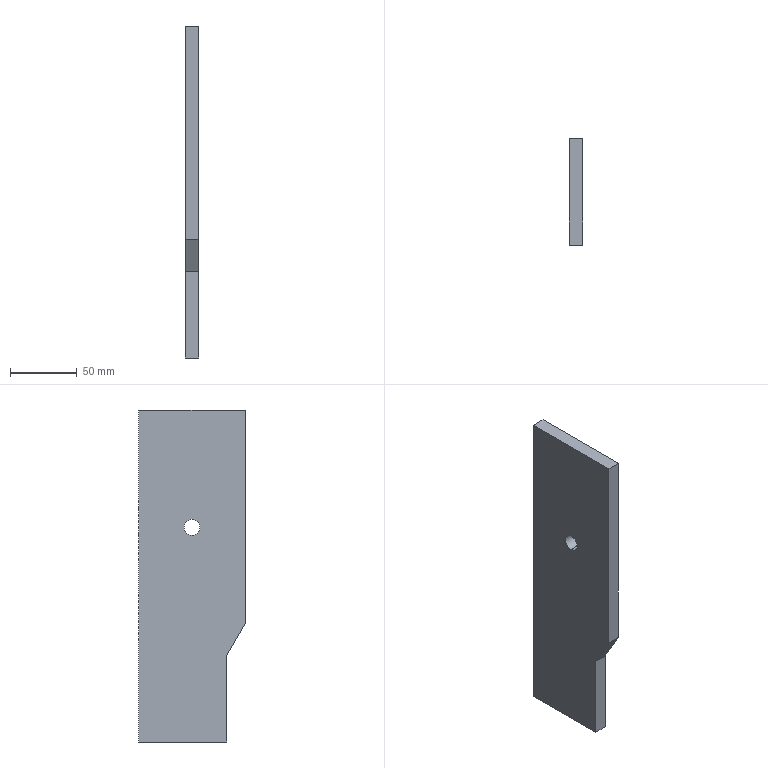Part | STEP file | VD-SYL0380DJ1006_1_4-3_VD-SYL03 | 1 solid | 10 faces | box 10 x 80 x 249 mm | volume 187272 mm3 | plane 8 | cylinder 2 | commonest cylinder face diameters 12 x2
STEP:
#1=CARTESIAN_POINT('',(0.,-40.,-94.));
#2=VERTEX_POINT('',#1);
#3=CARTESIAN_POINT('',(10.,-40.,-94.));
#4=VERTEX_POINT('',#3);
#5=CARTESIAN_POINT('',(0.,-40.,-94.));
#6=DIRECTION('',(1.,0.,0.));
#7=VECTOR('',#6,1000.);
#8=LINE('',#5,#7);
#9=EDGE_CURVE('',#2,#4,#8,.T.);
#10=ORIENTED_EDGE('',*,*,#9,.F.);
#11=CARTESIAN_POINT('',(0.,-40.,-82.));
#12=VERTEX_POINT('',#11);
#13=CARTESIAN_POINT('',(0.,-40.,-88.));
#14=DIRECTION('',(1.,0.,0.));
#15=DIRECTION('',(0.,0.,1.));
#16=AXIS2_PLACEMENT_3D('',#13,#14,#15);
#17=CIRCLE('',#16,6.);
#18=EDGE_CURVE('',#12,#2,#17,.T.);
#19=ORIENTED_EDGE('',*,*,#18,.F.);
#20=CARTESIAN_POINT('',(10.,-40.,-82.));
#21=VERTEX_POINT('',#20);
#22=CARTESIAN_POINT('',(0.,-40.,-82.));
#23=DIRECTION('',(1.,0.,0.));
#24=VECTOR('',#23,1000.);
#25=LINE('',#22,#24);
#26=EDGE_CURVE('',#12,#21,#25,.T.);
#27=ORIENTED_EDGE('',*,*,#26,.T.);
#28=CARTESIAN_POINT('',(10.,-40.,-88.));
#29=DIRECTION('',(-1.,0.,0.));
#30=DIRECTION('',(0.,0.,-1.));
#31=AXIS2_PLACEMENT_3D('',#28,#29,#30);
#32=CIRCLE('',#31,6.);
#33=EDGE_CURVE('',#4,#21,#32,.T.);
#34=ORIENTED_EDGE('',*,*,#33,.F.);
#35=EDGE_LOOP('',(#10,#19,#27,#34));
#36=FACE_OUTER_BOUND('',#35,.T.);
#37=CARTESIAN_POINT('',(0.,-40.,-88.));
#38=DIRECTION('',(-1.,0.,0.));
#39=DIRECTION('',(0.,0.,1.));
#40=AXIS2_PLACEMENT_3D('',#37,#38,#39);
#41=CYLINDRICAL_SURFACE('',#40,6.);
#42=ADVANCED_FACE('',(#36),#41,.F.);
#43=CARTESIAN_POINT('',(10.,-40.,-88.));
#44=DIRECTION('',(-1.,0.,0.));
#45=DIRECTION('',(0.,0.,1.));
#46=AXIS2_PLACEMENT_3D('',#43,#44,#45);
#47=CIRCLE('',#46,6.);
#48=EDGE_CURVE('',#21,#4,#47,.T.);
#49=ORIENTED_EDGE('',*,*,#48,.F.);
#50=ORIENTED_EDGE('',*,*,#26,.F.);
#51=CARTESIAN_POINT('',(0.,-40.,-88.));
#52=DIRECTION('',(1.,0.,0.));
#53=DIRECTION('',(0.,0.,-1.));
#54=AXIS2_PLACEMENT_3D('',#51,#52,#53);
#55=CIRCLE('',#54,6.);
#56=EDGE_CURVE('',#2,#12,#55,.T.);
#57=ORIENTED_EDGE('',*,*,#56,.F.);
#58=ORIENTED_EDGE('',*,*,#9,.T.);
#59=EDGE_LOOP('',(#49,#50,#57,#58));
#60=FACE_OUTER_BOUND('',#59,.T.);
#61=CARTESIAN_POINT('',(0.,-40.,-88.));
#62=DIRECTION('',(-1.,0.,0.));
#63=DIRECTION('',(0.,0.,1.));
#64=AXIS2_PLACEMENT_3D('',#61,#62,#63);
#65=CYLINDRICAL_SURFACE('',#64,6.);
#66=ADVANCED_FACE('',(#60),#65,.F.);
#67=ORIENTED_EDGE('',*,*,#33,.T.);
#68=ORIENTED_EDGE('',*,*,#48,.T.);
#69=EDGE_LOOP('',(#67,#68));
#70=FACE_BOUND('',#69,.T.);
#71=CARTESIAN_POINT('',(10.,0.,0.));
#72=VERTEX_POINT('',#71);
#73=CARTESIAN_POINT('',(10.,0.,-249.));
#74=VERTEX_POINT('',#73);
#75=CARTESIAN_POINT('',(10.,0.,0.));
#76=DIRECTION('',(0.,0.,-1.));
#77=VECTOR('',#76,1000.);
#78=LINE('',#75,#77);
#79=EDGE_CURVE('',#72,#74,#78,.T.);
#80=ORIENTED_EDGE('',*,*,#79,.F.);
#81=CARTESIAN_POINT('',(10.,-80.,0.));
#82=VERTEX_POINT('',#81);
#83=CARTESIAN_POINT('',(10.,-80.,0.));
#84=DIRECTION('',(0.,1.,0.));
#85=VECTOR('',#84,1000.);
#86=LINE('',#83,#85);
#87=EDGE_CURVE('',#82,#72,#86,.T.);
#88=ORIENTED_EDGE('',*,*,#87,.F.);
#89=CARTESIAN_POINT('',(10.,-80.,-159.751));
#90=VERTEX_POINT('',#89);
#91=CARTESIAN_POINT('',(10.,-80.,-159.751));
#92=DIRECTION('',(0.,0.,1.));
#93=VECTOR('',#92,1000.);
#94=LINE('',#91,#93);
#95=EDGE_CURVE('',#90,#82,#94,.T.);
#96=ORIENTED_EDGE('',*,*,#95,.F.);
#97=CARTESIAN_POINT('',(10.,-66.,-184.));
#98=VERTEX_POINT('',#97);
#99=CARTESIAN_POINT('',(10.,-80.,-159.751));
#100=DIRECTION('',(0.,0.5,-0.866));
#101=VECTOR('',#100,1000.);
#102=LINE('',#99,#101);
#103=EDGE_CURVE('',#90,#98,#102,.T.);
#104=ORIENTED_EDGE('',*,*,#103,.T.);
#105=CARTESIAN_POINT('',(10.,-66.,-249.));
#106=VERTEX_POINT('',#105);
#107=CARTESIAN_POINT('',(10.,-66.,-249.));
#108=DIRECTION('',(0.,0.,1.));
#109=VECTOR('',#108,1000.);
#110=LINE('',#107,#109);
#111=EDGE_CURVE('',#106,#98,#110,.T.);
#112=ORIENTED_EDGE('',*,*,#111,.F.);
#113=CARTESIAN_POINT('',(10.,0.,-249.));
#114=DIRECTION('',(0.,-1.,0.));
#115=VECTOR('',#114,1000.);
#116=LINE('',#113,#115);
#117=EDGE_CURVE('',#74,#106,#116,.T.);
#118=ORIENTED_EDGE('',*,*,#117,.F.);
#119=EDGE_LOOP('',(#80,#88,#96,#104,#112,#118));
#120=FACE_OUTER_BOUND('',#119,.T.);
#121=CARTESIAN_POINT('',(10.,0.,0.));
#122=DIRECTION('',(1.,0.,0.));
#123=DIRECTION('',(0.,1.,0.));
#124=AXIS2_PLACEMENT_3D('',#121,#122,#123);
#125=PLANE('',#124);
#126=ADVANCED_FACE('',(#70,#120),#125,.T.);
#127=CARTESIAN_POINT('',(0.,-66.,-184.));
#128=VERTEX_POINT('',#127);
#129=CARTESIAN_POINT('',(0.,-80.,-159.751));
#130=VERTEX_POINT('',#129);
#131=CARTESIAN_POINT('',(0.,-66.,-184.));
#132=DIRECTION('',(0.,-0.5,0.866));
#133=VECTOR('',#132,1000.);
#134=LINE('',#131,#133);
#135=EDGE_CURVE('',#128,#130,#134,.T.);
#136=ORIENTED_EDGE('',*,*,#135,.F.);
#137=CARTESIAN_POINT('',(0.,-66.,-184.));
#138=DIRECTION('',(1.,0.,0.));
#139=VECTOR('',#138,1000.);
#140=LINE('',#137,#139);
#141=EDGE_CURVE('',#128,#98,#140,.T.);
#142=ORIENTED_EDGE('',*,*,#141,.T.);
#143=ORIENTED_EDGE('',*,*,#103,.F.);
#144=CARTESIAN_POINT('',(0.,-80.,-159.751));
#145=DIRECTION('',(1.,0.,0.));
#146=VECTOR('',#145,1000.);
#147=LINE('',#144,#146);
#148=EDGE_CURVE('',#130,#90,#147,.T.);
#149=ORIENTED_EDGE('',*,*,#148,.F.);
#150=EDGE_LOOP('',(#136,#142,#143,#149));
#151=FACE_OUTER_BOUND('',#150,.T.);
#152=CARTESIAN_POINT('',(0.,-80.,-159.751));
#153=DIRECTION('',(0.,-0.866,-0.5));
#154=DIRECTION('',(0.,0.5,-0.866));
#155=AXIS2_PLACEMENT_3D('',#152,#153,#154);
#156=PLANE('',#155);
#157=ADVANCED_FACE('',(#151),#156,.T.);
#158=ORIENTED_EDGE('',*,*,#111,.T.);
#159=ORIENTED_EDGE('',*,*,#141,.F.);
#160=CARTESIAN_POINT('',(0.,-66.,-249.));
#161=VERTEX_POINT('',#160);
#162=CARTESIAN_POINT('',(0.,-66.,-249.));
#163=DIRECTION('',(0.,0.,1.));
#164=VECTOR('',#163,1000.);
#165=LINE('',#162,#164);
#166=EDGE_CURVE('',#161,#128,#165,.T.);
#167=ORIENTED_EDGE('',*,*,#166,.F.);
#168=CARTESIAN_POINT('',(0.,-66.,-249.));
#169=DIRECTION('',(1.,0.,0.));
#170=VECTOR('',#169,1000.);
#171=LINE('',#168,#170);
#172=EDGE_CURVE('',#161,#106,#171,.T.);
#173=ORIENTED_EDGE('',*,*,#172,.T.);
#174=EDGE_LOOP('',(#158,#159,#167,#173));
#175=FACE_OUTER_BOUND('',#174,.T.);
#176=CARTESIAN_POINT('',(0.,-66.,-184.));
#177=DIRECTION('',(0.,-1.,0.));
#178=DIRECTION('',(0.,0.,-1.));
#179=AXIS2_PLACEMENT_3D('',#176,#177,#178);
#180=PLANE('',#179);
#181=ADVANCED_FACE('',(#175),#180,.T.);
#182=CARTESIAN_POINT('',(0.,0.,-249.));
#183=VERTEX_POINT('',#182);
#184=CARTESIAN_POINT('',(0.,0.,-249.));
#185=DIRECTION('',(1.,0.,0.));
#186=VECTOR('',#185,1000.);
#187=LINE('',#184,#186);
#188=EDGE_CURVE('',#183,#74,#187,.T.);
#189=ORIENTED_EDGE('',*,*,#188,.T.);
#190=ORIENTED_EDGE('',*,*,#117,.T.);
#191=ORIENTED_EDGE('',*,*,#172,.F.);
#192=CARTESIAN_POINT('',(0.,0.,-249.));
#193=DIRECTION('',(0.,-1.,0.));
#194=VECTOR('',#193,1000.);
#195=LINE('',#192,#194);
#196=EDGE_CURVE('',#183,#161,#195,.T.);
#197=ORIENTED_EDGE('',*,*,#196,.F.);
#198=EDGE_LOOP('',(#189,#190,#191,#197));
#199=FACE_OUTER_BOUND('',#198,.T.);
#200=CARTESIAN_POINT('',(0.,0.,-249.));
#201=DIRECTION('',(0.,0.,-1.));
#202=DIRECTION('',(0.,-1.,0.));
#203=AXIS2_PLACEMENT_3D('',#200,#201,#202);
#204=PLANE('',#203);
#205=ADVANCED_FACE('',(#199),#204,.T.);
#206=CARTESIAN_POINT('',(0.,0.,0.));
#207=VERTEX_POINT('',#206);
#208=CARTESIAN_POINT('',(0.,0.,0.));
#209=DIRECTION('',(0.,0.,-1.));
#210=VECTOR('',#209,1000.);
#211=LINE('',#208,#210);
#212=EDGE_CURVE('',#207,#183,#211,.T.);
#213=ORIENTED_EDGE('',*,*,#212,.F.);
#214=CARTESIAN_POINT('',(10.,0.,0.));
#215=DIRECTION('',(-1.,0.,0.));
#216=VECTOR('',#215,1000.);
#217=LINE('',#214,#216);
#218=EDGE_CURVE('',#72,#207,#217,.T.);
#219=ORIENTED_EDGE('',*,*,#218,.F.);
#220=ORIENTED_EDGE('',*,*,#79,.T.);
#221=ORIENTED_EDGE('',*,*,#188,.F.);
#222=EDGE_LOOP('',(#213,#219,#220,#221));
#223=FACE_OUTER_BOUND('',#222,.T.);
#224=CARTESIAN_POINT('',(0.,0.,-239.));
#225=DIRECTION('',(0.,1.,0.));
#226=DIRECTION('',(1.,0.,0.));
#227=AXIS2_PLACEMENT_3D('',#224,#225,#226);
#228=PLANE('',#227);
#229=ADVANCED_FACE('',(#223),#228,.T.);
#230=CARTESIAN_POINT('',(0.,-80.,0.));
#231=VERTEX_POINT('',#230);
#232=CARTESIAN_POINT('',(0.,-80.,0.));
#233=DIRECTION('',(0.,1.,0.));
#234=VECTOR('',#233,1000.);
#235=LINE('',#232,#234);
#236=EDGE_CURVE('',#231,#207,#235,.T.);
#237=ORIENTED_EDGE('',*,*,#236,.F.);
#238=CARTESIAN_POINT('',(0.,-80.,0.));
#239=DIRECTION('',(1.,0.,0.));
#240=VECTOR('',#239,1000.);
#241=LINE('',#238,#240);
#242=EDGE_CURVE('',#231,#82,#241,.T.);
#243=ORIENTED_EDGE('',*,*,#242,.T.);
#244=ORIENTED_EDGE('',*,*,#87,.T.);
#245=ORIENTED_EDGE('',*,*,#218,.T.);
#246=EDGE_LOOP('',(#237,#243,#244,#245));
#247=FACE_OUTER_BOUND('',#246,.T.);
#248=CARTESIAN_POINT('',(0.,0.,0.));
#249=DIRECTION('',(0.,0.,1.));
#250=DIRECTION('',(1.,0.,0.));
#251=AXIS2_PLACEMENT_3D('',#248,#249,#250);
#252=PLANE('',#251);
#253=ADVANCED_FACE('',(#247),#252,.T.);
#254=CARTESIAN_POINT('',(0.,-80.,-159.751));
#255=DIRECTION('',(0.,0.,1.));
#256=VECTOR('',#255,1000.);
#257=LINE('',#254,#256);
#258=EDGE_CURVE('',#130,#231,#257,.T.);
#259=ORIENTED_EDGE('',*,*,#258,.F.);
#260=ORIENTED_EDGE('',*,*,#148,.T.);
#261=ORIENTED_EDGE('',*,*,#95,.T.);
#262=ORIENTED_EDGE('',*,*,#242,.F.);
#263=EDGE_LOOP('',(#259,#260,#261,#262));
#264=FACE_OUTER_BOUND('',#263,.T.);
#265=CARTESIAN_POINT('',(0.,-80.,0.));
#266=DIRECTION('',(0.,-1.,0.));
#267=DIRECTION('',(0.,0.,-1.));
#268=AXIS2_PLACEMENT_3D('',#265,#266,#267);
#269=PLANE('',#268);
#270=ADVANCED_FACE('',(#264),#269,.T.);
#271=ORIENTED_EDGE('',*,*,#56,.T.);
#272=ORIENTED_EDGE('',*,*,#18,.T.);
#273=EDGE_LOOP('',(#271,#272));
#274=FACE_BOUND('',#273,.T.);
#275=ORIENTED_EDGE('',*,*,#236,.T.);
#276=ORIENTED_EDGE('',*,*,#212,.T.);
#277=ORIENTED_EDGE('',*,*,#196,.T.);
#278=ORIENTED_EDGE('',*,*,#166,.T.);
#279=ORIENTED_EDGE('',*,*,#135,.T.);
#280=ORIENTED_EDGE('',*,*,#258,.T.);
#281=EDGE_LOOP('',(#275,#276,#277,#278,#279,#280));
#282=FACE_OUTER_BOUND('',#281,.T.);
#283=CARTESIAN_POINT('',(0.,0.,0.));
#284=DIRECTION('',(1.,0.,0.));
#285=DIRECTION('',(0.,1.,0.));
#286=AXIS2_PLACEMENT_3D('',#283,#284,#285);
#287=PLANE('',#286);
#288=ADVANCED_FACE('',(#274,#282),#287,.F.);
#289=CLOSED_SHELL('',(#42,#66,#126,#157,#181,#205,#229,#253,#270,#288));
#290=MANIFOLD_SOLID_BREP('',#289);
#291=CARTESIAN_POINT('',(0.,0.,0.));
#292=DIRECTION('',(0.,0.,1.));
#293=DIRECTION('',(1.,0.,0.));
#294=AXIS2_PLACEMENT_3D('',#291,#292,#293);
#295=(LENGTH_UNIT()NAMED_UNIT(*)SI_UNIT(.MILLI.,.METRE.));
#296=UNCERTAINTY_MEASURE_WITH_UNIT(LENGTH_MEASURE(0.00001),#295,'','');
#297=(NAMED_UNIT(*)PLANE_ANGLE_UNIT()SI_UNIT($,.RADIAN.));
#298=(NAMED_UNIT(*)SI_UNIT($,.STERADIAN.)SOLID_ANGLE_UNIT());
#299=(GEOMETRIC_REPRESENTATION_CONTEXT(3)GLOBAL_UNCERTAINTY_ASSIGNED_CONTEXT((#296))GLOBAL_UNIT_ASSIGNED_CONTEXT((#295,#297,#298))REPRESENTATION_CONTEXT('',''));
#300=ADVANCED_BREP_SHAPE_REPRESENTATION('',(#290,#294),#299);